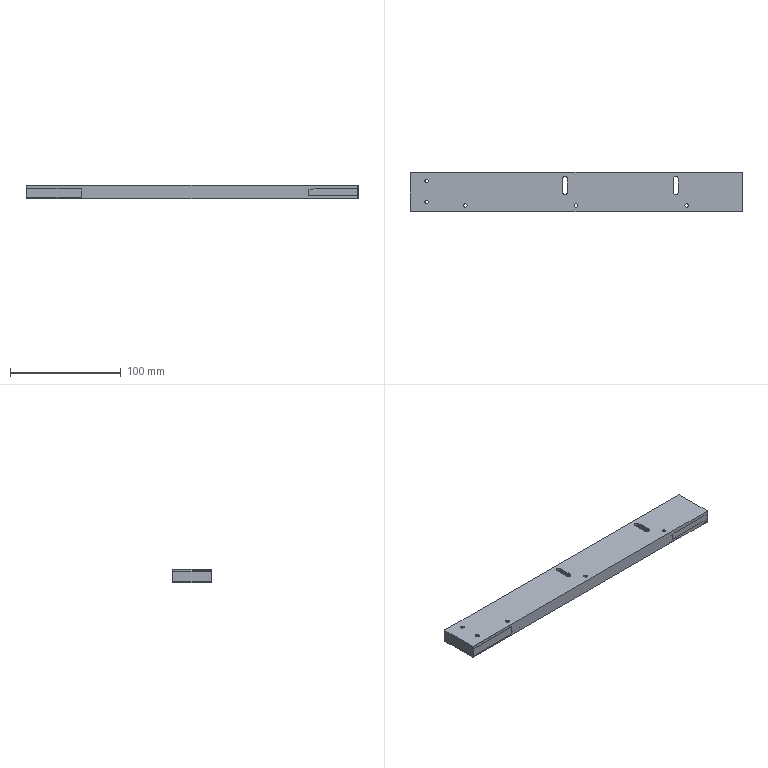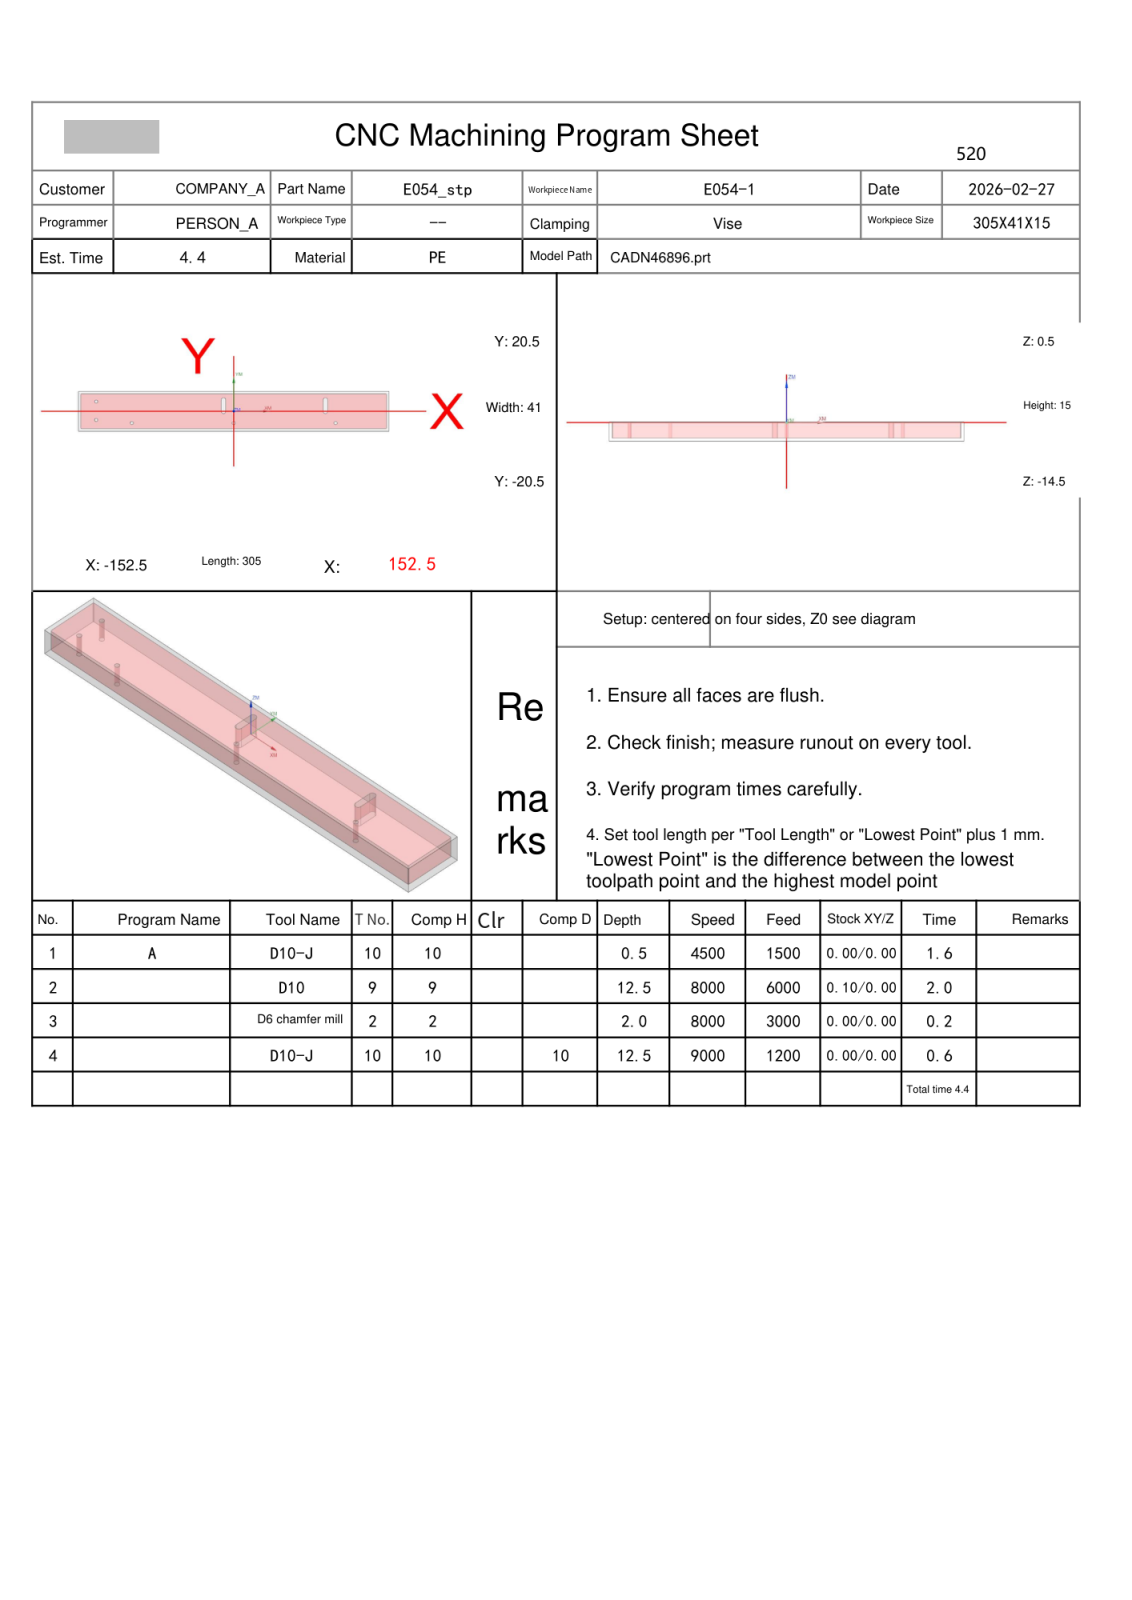NC program | NX | posted by the shop | part box 300 x 36 x 12 mm
Whole program:
%
O0001
(Machine time: 5.27 MIN)
(===Total Tool:3===)
(T10=D10-J  D=10.  R=0.   D-  H10 Z=-12.  )
(T9=D10     D=10.  R=0.   D-  H09 Z=-12.  )
(T2=D6 chamfer mill   D=6.   R=0.   D-  H02 Z=-1.5  )
G80 G90 G17 G49 G40
G91 G28 Z0
M01
N1 T10 M06
(D10-J  D=10. R=0. H=10 ce=0.00 di=0.00)
G00 G90 G54 X-160. Y8.111 M03 S4500
G43 H10 Z50.
M08
Z2.
G01 Z0.0 F1500.
X-155. Y13.111
X-145.111 Y23.
X-135.222
X-155. Y3.222
Y-6.667
X-125.333 Y23.
X-115.444
X-155. Y-16.556
Y-23.
X-151.556
X-105.556 Y23.
X-95.667
X-141.667 Y-23.
X-131.778
X-85.778 Y23.
X-75.889
X-121.889 Y-23.
X-112.
X-66. Y23.
X-56.111
X-102.111 Y-23.
X-92.222
X-46.222 Y23.
X-36.333
X-82.333 Y-23.
X-72.444
X-26.444 Y23.
X-16.556
X-62.556 Y-23.
X-52.667
X-6.667 Y23.
X3.222
X-42.778 Y-23.
X-32.889
X13.111 Y23.
X23.
X-23. Y-23.
X-13.111
X32.889 Y23.
X42.778
X-3.222 Y-23.
X6.667
X52.667 Y23.
X62.556
X16.556 Y-23.
X26.444
X72.444 Y23.
X82.333
X36.333 Y-23.
X46.222
X92.222 Y23.
X102.111
X56.111 Y-23.
X66.
X112. Y23.
X121.889
X75.889 Y-23.
X85.778
X131.778 Y23.
X141.667
X95.667 Y-23.
X105.556
X151.556 Y23.
X155.
Y16.556
X115.444 Y-23.
X125.333
X155. Y6.667
Y-3.222
X135.222 Y-23.
X145.111
X155. Y-13.111
X160. Y-8.111
Z2.
G00 Z50.
G91 G28 Z0.0
M05
M09
G91 G28 Z0.0
M01
N2 T09 M06
(D10  D=10. R=0. H=09 ce=0.10 di=0.00)
G00 G90 G54 X0.0 Y-23.1 M03 S8000
G43 H09 Z50.
M08
Z.5
G01 X-149.5 Z.334 F6000.
G02 X-153.106 Y-21.606 Z.329 I0.0 J5.1
G01 X-153.606 Y-21.106
G02 X-155.1 Y-17.5 Z.324 I3.606 J3.606
G01 Y17.5 Z.285
G02 X-153.606 Y21.106 Z.281 I5.1 J0.0
G01 X-153.106 Y21.606 Z.28
G02 X-149.5 Y23.1 Z.276 I3.606 J-3.606
G01 X149.5 Z-.057
G02 X153.106 Y21.606 Z-.061 I0.0 J-5.1
G01 X153.606 Y21.106 Z-.062
G02 X155.1 Y17.5 Z-.066 I-3.606 J-3.606
G01 Y-17.5 Z-.105
G02 X153.606 Y-21.106 Z-.11 I-5.1 J0.0
G01 X153.106 Y-21.606 Z-.111
G02 X149.5 Y-23.1 Z-.115 I-3.606 J3.606
G01 X-149.5 Z-.447
G02 X-153.106 Y-21.606 Z-.452 I0.0 J5.1
G01 X-153.606 Y-21.106 Z-.453
G02 X-155.1 Y-17.5 Z-.457 I3.606 J3.606
G01 Y17.5 Z-.496
G02 X-153.606 Y21.106 Z-.5 I5.1 J0.0
G01 X-153.106 Y21.606 Z-.501
G02 X-149.5 Y23.1 Z-.506 I3.606 J-3.606
G01 X149.5 Z-.838
G02 X153.106 Y21.606 Z-.842 I0.0 J-5.1
G01 X153.606 Y21.106 Z-.843
G02 X155.1 Y17.5 Z-.848 I-3.606 J-3.606
G01 Y-17.5 Z-.887
G02 X153.606 Y-21.106 Z-.891 I-5.1 J0.0
G01 X153.106 Y-21.606 Z-.892
G02 X149.5 Y-23.1 Z-.896 I-3.606 J3.606
G01 X-149.5 Z-1.229
G02 X-153.106 Y-21.606 Z-1.233 I0.0 J5.1
G01 X-153.606 Y-21.106 Z-1.234
G02 X-155.1 Y-17.5 Z-1.238 I3.606 J3.606
G01 Y17.5 Z-1.277
G02 X-153.606 Y21.106 Z-1.282 I5.1 J0.0
G01 X-153.106 Y21.606 Z-1.283
G02 X-149.5 Y23.1 Z-1.287 I3.606 J-3.606
G01 X149.5 Z-1.619
G02 X153.106 Y21.606 Z-1.624 I0.0 J-5.1
G01 X153.606 Y21.106 Z-1.625
G02 X155.1 Y17.5 Z-1.629 I-3.606 J-3.606
G01 Y-17.5 Z-1.668
G02 X153.606 Y-21.106 Z-1.672 I-5.1 J0.0
G01 X153.106 Y-21.606 Z-1.673
G02 X149.5 Y-23.1 Z-1.678 I-3.606 J3.606
G01 X-149.5 Z-2.01
G02 X-153.106 Y-21.606 Z-2.014 I0.0 J5.1
G01 X-153.606 Y-21.106 Z-2.015
G02 X-155.1 Y-17.5 Z-2.02 I3.606 J3.606
G01 Y17.5 Z-2.059
G02 X-153.606 Y21.106 Z-2.063 I5.1 J0.0
G01 X-153.106 Y21.606 Z-2.064
G02 X-149.5 Y23.1 Z-2.068 I3.606 J-3.606
G01 X149.5 Z-2.401
G02 X153.106 Y21.606 Z-2.405 I0.0 J-5.1
G01 X153.606 Y21.106 Z-2.406
G02 X155.1 Y17.5 Z-2.41 I-3.606 J-3.606
G01 Y-17.5 Z-2.449
G02 X153.606 Y-21.106 Z-2.454 I-5.1 J0.0
G01 X153.106 Y-21.606
G02 X149.5 Y-23.1 Z-2.459 I-3.606 J3.606
G01 X-149.5 Z-2.791
G02 X-153.106 Y-21.606 Z-2.796 I0.0 J5.1
G01 X-153.606 Y-21.106
G02 X-155.1 Y-17.5 Z-2.801 I3.606 J3.606
G01 Y17.5 Z-2.84
G02 X-153.606 Y21.106 Z-2.844 I5.1 J0.0
G01 X-153.106 Y21.606 Z-2.845
G02 X-149.5 Y23.1 Z-2.849 I3.606 J-3.606
G01 X149.5 Z-3.182
G02 X153.106 Y21.606 Z-3.186 I0.0 J-5.1
G01 X153.606 Y21.106 Z-3.187
G02 X155.1 Y17.5 Z-3.191 I-3.606 J-3.606
G01 Y-17.5 Z-3.23
G02 X153.606 Y-21.106 Z-3.235 I-5.1 J0.0
G01 X153.106 Y-21.606 Z-3.236
G02 X149.5 Y-23.1 Z-3.24 I-3.606 J3.606
G01 X-149.5 Z-3.572
G02 X-153.106 Y-21.606 Z-3.577 I0.0 J5.1
G01 X-153.606 Y-21.106 Z-3.578
G02 X-155.1 Y-17.5 Z-3.582 I3.606 J3.606
G01 Y17.5 Z-3.621
G02 X-153.606 Y21.106 Z-3.625 I5.1 J0.0
G01 X-153.106 Y21.606 Z-3.626
G02 X-149.5 Y23.1 Z-3.631 I3.606 J-3.606
G01 X149.5 Z-3.963
G02 X153.106 Y21.606 Z-3.967 I0.0 J-5.1
G01 X153.606 Y21.106 Z-3.968
G02 X155.1 Y17.5 Z-3.973 I-3.606 J-3.606
G01 Y-17.5 Z-4.012
G02 X153.606 Y-21.106 Z-4.016 I-5.1 J0.0
G01 X153.106 Y-21.606 Z-4.017
G02 X149.5 Y-23.1 Z-4.021 I-3.606 J3.606
G01 X-149.5 Z-4.354
G02 X-153.106 Y-21.606 Z-4.358 I0.0 J5.1
G01 X-153.606 Y-21.106 Z-4.359
G02 X-155.1 Y-17.5 Z-4.363 I3.606 J3.606
G01 Y17.5 Z-4.402
G02 X-153.606 Y21.106 Z-4.407 I5.1 J0.0
G01 X-153.106 Y21.606 Z-4.408
G02 X-149.5 Y23.1 Z-4.412 I3.606 J-3.606
G01 X149.5 Z-4.744
G02 X153.106 Y21.606 Z-4.749 I0.0 J-5.1
G01 X153.606 Y21.106 Z-4.75
G02 X155.1 Y17.5 Z-4.754 I-3.606 J-3.606
G01 Y-17.5 Z-4.793
G02 X153.606 Y-21.106 Z-4.797 I-5.1 J0.0
G01 X153.106 Y-21.606 Z-4.798
G02 X149.5 Y-23.1 Z-4.803 I-3.606 J3.606
G01 X-149.5 Z-5.135
G02 X-153.106 Y-21.606 Z-5.139 I0.0 J5.1
G01 X-153.606 Y-21.106 Z-5.14
G02 X-155.1 Y-17.5 Z-5.145 I3.606 J3.606
G01 Y17.5 Z-5.184
G02 X-153.606 Y21.106 Z-5.188 I5.1 J0.0
G01 X-153.106 Y21.606 Z-5.189
G02 X-149.5 Y23.1 Z-5.193 I3.606 J-3.606
G01 X149.5 Z-5.526
G02 X153.106 Y21.606 Z-5.53 I0.0 J-5.1
G01 X153.606 Y21.106 Z-5.531
G02 X155.1 Y17.5 Z-5.535 I-3.606 J-3.606
G01 Y-17.5 Z-5.574
G02 X153.606 Y-21.106 Z-5.579 I-5.1 J0.0
G01 X153.106 Y-21.606
G02 X149.5 Y-23.1 Z-5.584 I-3.606 J3.606
G01 X-149.5 Z-5.916
G02 X-153.106 Y-21.606 Z-5.921 I0.0 J5.1
G01 X-153.606 Y-21.106
G02 X-155.1 Y-17.5 Z-5.926 I3.606 J3.606
G01 Y17.5 Z-5.965
G02 X-153.606 Y21.106 Z-5.969 I5.1 J0.0
G01 X-153.106 Y21.606 Z-5.97
G02 X-149.5 Y23.1 Z-5.974 I3.606 J-3.606
G01 X149.5 Z-6.307
G02 X153.106 Y21.606 Z-6.311 I0.0 J-5.1
G01 X153.606 Y21.106 Z-6.312
G02 X155.1 Y17.5 Z-6.316 I-3.606 J-3.606
G01 Y-17.5 Z-6.355
G02 X153.606 Y-21.106 Z-6.36 I-5.1 J0.0
G01 X153.106 Y-21.606 Z-6.361
G02 X149.5 Y-23.1 Z-6.365 I-3.606 J3.606
G01 X-149.5 Z-6.697
G02 X-153.106 Y-21.606 Z-6.702 I0.0 J5.1
G01 X-153.606 Y-21.106 Z-6.703
G02 X-155.1 Y-17.5 Z-6.707 I3.606 J3.606
G01 Y17.5 Z-6.746
G02 X-153.606 Y21.106 Z-6.75 I5.1 J0.0
G01 X-153.106 Y21.606 Z-6.751
G02 X-149.5 Y23.1 Z-6.756 I3.606 J-3.606
G01 X149.5 Z-7.088
G02 X153.106 Y21.606 Z-7.092 I0.0 J-5.1
G01 X153.606 Y21.106 Z-7.093
G02 X155.1 Y17.5 Z-7.098 I-3.606 J-3.606
G01 Y-17.5 Z-7.137
G02 X153.606 Y-21.106 Z-7.141 I-5.1 J0.0
G01 X153.106 Y-21.606 Z-7.142
G02 X149.5 Y-23.1 Z-7.146 I-3.606 J3.606
G01 X-149.5 Z-7.479
G02 X-153.106 Y-21.606 Z-7.483 I0.0 J5.1
G01 X-153.606 Y-21.106 Z-7.484
G02 X-155.1 Y-17.5 Z-7.488 I3.606 J3.606
G01 Y17.5 Z-7.527
G02 X-153.606 Y21.106 Z-7.532 I5.1 J0.0
G01 X-153.106 Y21.606 Z-7.533
G02 X-149.5 Y23.1 Z-7.537 I3.606 J-3.606
G01 X149.5 Z-7.869
G02 X153.106 Y21.606 Z-7.874 I0.0 J-5.1
G01 X153.606 Y21.106 Z-7.875
G02 X155.1 Y17.5 Z-7.879 I-3.606 J-3.606
G01 Y-17.5 Z-7.918
G02 X153.606 Y-21.106 Z-7.922 I-5.1 J0.0
G01 X153.106 Y-21.606 Z-7.923
G02 X149.5 Y-23.1 Z-7.928 I-3.606 J3.606
G01 X-149.5 Z-8.26
G02 X-153.106 Y-21.606 Z-8.264 I0.0 J5.1
G01 X-153.606 Y-21.106 Z-8.265
G02 X-155.1 Y-17.5 Z-8.27 I3.606 J3.606
G01 Y17.5 Z-8.309
G02 X-153.606 Y21.106 Z-8.313 I5.1 J0.0
G01 X-153.106 Y21.606 Z-8.314
G02 X-149.5 Y23.1 Z-8.318 I3.606 J-3.606
G01 X149.5 Z-8.651
G02 X153.106 Y21.606 Z-8.655 I0.0 J-5.1
G01 X153.606 Y21.106 Z-8.656
G02 X155.1 Y17.5 Z-8.66 I-3.606 J-3.606
G01 Y-17.5 Z-8.699
G02 X153.606 Y-21.106 Z-8.704 I-5.1 J0.0
G01 X153.106 Y-21.606
G02 X149.5 Y-23.1 Z-8.709 I-3.606 J3.606
G01 X-149.5 Z-9.041
G02 X-153.106 Y-21.606 Z-9.046 I0.0 J5.1
G01 X-153.606 Y-21.106
G02 X-155.1 Y-17.5 Z-9.051 I3.606 J3.606
G01 Y17.5 Z-9.09
G02 X-153.606 Y21.106 Z-9.094 I5.1 J0.0
G01 X-153.106 Y21.606 Z-9.095
G02 X-149.5 Y23.1 Z-9.099 I3.606 J-3.606
G01 X149.5 Z-9.432
G02 X153.106 Y21.606 Z-9.436 I0.0 J-5.1
G01 X153.606 Y21.106 Z-9.437
G02 X155.1 Y17.5 Z-9.441 I-3.606 J-3.606
G01 Y-17.5 Z-9.48
G02 X153.606 Y-21.106 Z-9.485 I-5.1 J0.0
G01 X153.106 Y-21.606 Z-9.486
G02 X149.5 Y-23.1 Z-9.49 I-3.606 J3.606
G01 X-149.5 Z-9.822
G02 X-153.106 Y-21.606 Z-9.827 I0.0 J5.1
G01 X-153.606 Y-21.106 Z-9.828
G02 X-155.1 Y-17.5 Z-9.832 I3.606 J3.606
G01 Y17.5 Z-9.871
G02 X-153.606 Y21.106 Z-9.875 I5.1 J0.0
G01 X-153.106 Y21.606 Z-9.876
G02 X-149.5 Y23.1 Z-9.881 I3.606 J-3.606
G01 X149.5 Z-10.213
G02 X153.106 Y21.606 Z-10.217 I0.0 J-5.1
G01 X153.606 Y21.106 Z-10.218
G02 X155.1 Y17.5 Z-10.223 I-3.606 J-3.606
G01 Y-17.5 Z-10.262
G02 X153.606 Y-21.106 Z-10.266 I-5.1 J0.0
G01 X153.106 Y-21.606 Z-10.267
G02 X149.5 Y-23.1 Z-10.271 I-3.606 J3.606
G01 X-149.5 Z-10.604
G02 X-153.106 Y-21.606 Z-10.608 I0.0 J5.1
G01 X-153.606 Y-21.106 Z-10.609
G02 X-155.1 Y-17.5 Z-10.613 I3.606 J3.606
G01 Y17.5 Z-10.652
G02 X-153.606 Y21.106 Z-10.657 I5.1 J0.0
G01 X-153.106 Y21.606 Z-10.658
G02 X-149.5 Y23.1 Z-10.662 I3.606 J-3.606
G01 X149.5 Z-10.994
G02 X153.106 Y21.606 Z-10.999 I0.0 J-5.1
G01 X153.606 Y21.106 Z-11.
G02 X155.1 Y17.5 Z-11.004 I-3.606 J-3.606
G01 Y-17.5 Z-11.043
G02 X153.606 Y-21.106 Z-11.047 I-5.1 J0.0
G01 X153.106 Y-21.606 Z-11.048
G02 X149.5 Y-23.1 Z-11.053 I-3.606 J3.606
G01 X-149.5 Z-11.385
G02 X-153.106 Y-21.606 Z-11.389 I0.0 J5.1
G01 X-153.606 Y-21.106 Z-11.39
G02 X-155.1 Y-17.5 Z-11.395 I3.606 J3.606
G01 Y17.5 Z-11.434
G02 X-153.606 Y21.106 Z-11.438 I5.1 J0.0
G01 X-153.106 Y21.606 Z-11.439
G02 X-149.5 Y23.1 Z-11.443 I3.606 J-3.606
G01 X149.5 Z-11.776
G02 X153.106 Y21.606 Z-11.78 I0.0 J-5.1
G01 X153.606 Y21.106 Z-11.781
G02 X155.1 Y17.5 Z-11.785 I-3.606 J-3.606
G01 Y-17.5 Z-11.824
G02 X153.606 Y-21.106 Z-11.829 I-5.1 J0.0
G01 X153.106 Y-21.606
G02 X149.5 Y-23.1 Z-11.834 I-3.606 J3.606
G01 X0.0 Z-12.
X-149.5
G02 X-153.106 Y-21.606 I0.0 J5.1
G01 X-153.606 Y-21.106
G02 X-155.1 Y-17.5 I3.606 J3.606
G01 Y17.5
G02 X-153.606 Y21.106 I5.1 J0.0
G01 X-153.106 Y21.606
G02 X-149.5 Y23.1 I3.606 J-3.606
G01 X149.5
G02 X153.106 Y21.606 I0.0 J-5.1
G01 X153.606 Y21.106
G02 X155.1 Y17.5 I-3.606 J-3.606
G01 Y-17.5
G02 X153.606 Y-21.106 I-5.1 J0.0
G01 X153.106 Y-21.606
G02 X149.5 Y-23.1 I-3.606 J3.606
G01 X0.0
X-.5
Z-11.
G00 Z50.
G91 G28 Z0.0
M05
M09
G91 G28 Z0.0
M01
N3 T02 M06
(D6 chamfer mill  D=6. R=0. H=02 ce=0.00 di=0.00)
G00 G90 G54 X-.25 Y20.128 M03 S8000
G43 H02 Z50.
M08
Z2.099
G01 Z-1.5 F3000.
G03 X-.33 Y19.828 I.52 J-.3
X-.03 Y19.308 I.6 J0.0
G01 X0.0 Y19.3
X149.5
X149.754 Y19.275
X149.997 Y19.201
X150.222 Y19.081
X150.419 Y18.919
X150.919 Y18.419
X151.081 Y18.222
X151.201 Y17.997
X151.275 Y17.754
X151.3 Y17.5
Y-17.5
X151.275 Y-17.754
X151.201 Y-17.997
X151.081 Y-18.222
X150.919 Y-18.419
X150.419 Y-18.919
X150.222 Y-19.081
X149.997 Y-19.201
X149.754 Y-19.275
X149.5 Y-19.3
X-149.5
X-149.754 Y-19.275
X-149.997 Y-19.201
X-150.222 Y-19.081
X-150.419 Y-18.919
X-150.919 Y-18.419
X-151.081 Y-18.222
X-151.201 Y-17.997
X-151.275 Y-17.754
X-151.3 Y-17.5
Y17.5
X-151.275 Y17.754
X-151.201 Y17.997
X-151.081 Y18.222
X-150.919 Y18.419
X-150.419 Y18.919
X-150.222 Y19.081
X-149.997 Y19.201
X-149.754 Y19.275
X-149.5 Y19.3
X0.0
X.03 Y19.308
G03 X.33 Y19.828 I-.3 J.52
X.25 Y20.128 I-.6 J0.0
G01 Z2.099
G00 Z50.
G91 G28 Z0.0
M05
M09
G91 G28 Z0.0
M01
N4 T10 M06
(D10-J  D=10. R=0. H=10 ce=0.00 di=0.00)
G00 G90 G54 X150.513 Y-24.116 M03 S9000
G43 H10 Z50.
M08
Z-11.5
G01 Z-12. F1200.
G41 D10
X150.497 Y-23.917
G03 X149.5 Y-23. I-.997 J-.083
G01 X-149.5
G02 X-153.036 Y-21.536 I0.0 J5.
G01 X-153.536 Y-21.036
G02 X-155. Y-17.5 I3.536 J3.536
G01 Y17.5
G02 X-153.536 Y21.036 I5. J0.0
G01 X-153.036 Y21.536
G02 X-149.5 Y23. I3.536 J-3.536
G01 X149.5
G02 X153.036 Y21.536 I0.0 J-5.
G01 X153.536 Y21.036
G02 X155. Y17.5 I-3.536 J-3.536
G01 Y-17.5
G02 X153.536 Y-21.036 I-5. J0.0
G01 X153.036 Y-21.536
G02 X149.5 Y-23. I-3.536 J3.536
G01 X149.
G03 X148. Y-24. I0.0 J-1.
G01 G40 Y-24.2
Z-11.5
G00 Z50.
M05
M09
G91 G28 Z0.0
G91 G28 Y0.0
M30
%